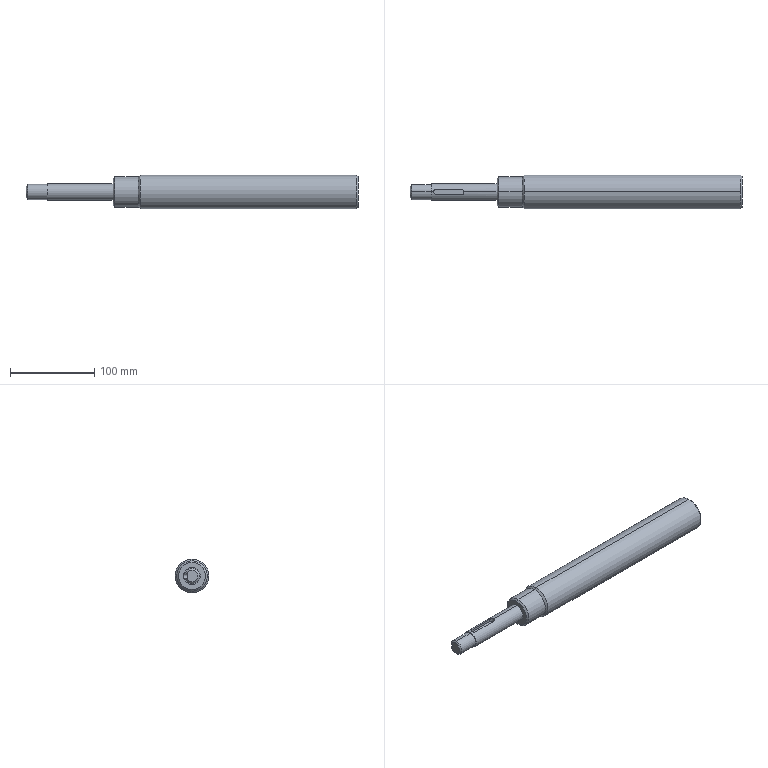Part | SolidWorks | features ICE 2, Chamfer 1, Revolution 1 | 1 solid | 32 faces | box 393 x 40 x 40 mm | volume 386098 mm3 | cylinder 13 | plane 10 | cone 9 | commonest cylinder face diameters 6 x3 18 x3 20 x2 36 x2 40 x2 5 x1
STEP:
#1=CARTESIAN_POINT('',(28.,0.,10.));
#2=VERTEX_POINT('',#1);
#3=CARTESIAN_POINT('',(31.,3.,9.539));
#4=VERTEX_POINT('',#3);
#5=CARTESIAN_POINT('',(28.,0.,10.));
#6=CARTESIAN_POINT('',(28.,0.1968,10.));
#7=CARTESIAN_POINT('',(28.02,0.3967,9.994));
#8=CARTESIAN_POINT('',(28.097,0.7821,9.971));
#9=CARTESIAN_POINT('',(28.154,0.9695,9.955));
#10=CARTESIAN_POINT('',(28.306,1.334,9.912));
#11=CARTESIAN_POINT('',(28.399,1.507,9.887));
#12=CARTESIAN_POINT('',(28.616,1.831,9.832));
#13=CARTESIAN_POINT('',(28.741,1.983,9.802));
#14=CARTESIAN_POINT('',(29.017,2.26,9.742));
#15=CARTESIAN_POINT('',(29.167,2.383,9.713));
#16=CARTESIAN_POINT('',(29.491,2.6,9.657));
#17=CARTESIAN_POINT('',(29.667,2.694,9.63));
#18=CARTESIAN_POINT('',(30.028,2.845,9.587));
#19=CARTESIAN_POINT('',(30.215,2.902,9.57));
#20=CARTESIAN_POINT('',(30.601,2.98,9.546));
#21=CARTESIAN_POINT('',(30.801,3.,9.539));
#22=CARTESIAN_POINT('',(31.,3.,9.539));
#23=B_SPLINE_CURVE_WITH_KNOTS('',3,(#5,#6,#7,#8,#9,#10,#11,#12,#13,#14,#15,#16,#17,#18,#19,#20,#21,#22),.UNSPECIFIED.,.F.,.F.,(4,2,2,2,2,2,2,2,4),(0.004718,0.005307,0.005896,0.006485,0.007074,0.007663,0.008252,0.008842,0.009431),.UNSPECIFIED.);
#24=EDGE_CURVE('',#2,#4,#23,.T.);
#25=ORIENTED_EDGE('',*,*,#24,.F.);
#26=CARTESIAN_POINT('',(28.,0.,6.5));
#27=VERTEX_POINT('',#26);
#28=CARTESIAN_POINT('',(28.,0.,20.001));
#29=DIRECTION('',(0.,0.,-1.));
#30=VECTOR('',#29,1000.);
#31=LINE('',#28,#30);
#32=EDGE_CURVE('',#2,#27,#31,.T.);
#33=ORIENTED_EDGE('',*,*,#32,.T.);
#34=CARTESIAN_POINT('',(31.,3.,6.5));
#35=VERTEX_POINT('',#34);
#36=CARTESIAN_POINT('',(31.,0.,6.5));
#37=DIRECTION('',(0.,0.,1.));
#38=DIRECTION('',(1.,0.,0.));
#39=AXIS2_PLACEMENT_3D('',#36,#37,#38);
#40=CIRCLE('',#39,3.);
#41=EDGE_CURVE('',#35,#27,#40,.T.);
#42=ORIENTED_EDGE('',*,*,#41,.F.);
#43=CARTESIAN_POINT('',(31.,3.,20.001));
#44=DIRECTION('',(0.,0.,-1.));
#45=VECTOR('',#44,1000.);
#46=LINE('',#43,#45);
#47=EDGE_CURVE('',#4,#35,#46,.T.);
#48=ORIENTED_EDGE('',*,*,#47,.F.);
#49=EDGE_LOOP('',(#25,#33,#42,#48));
#50=FACE_OUTER_BOUND('',#49,.T.);
#51=CARTESIAN_POINT('',(31.,0.,20.001));
#52=DIRECTION('',(0.,0.,-1.));
#53=DIRECTION('',(-1.,0.,0.));
#54=AXIS2_PLACEMENT_3D('',#51,#52,#53);
#55=CYLINDRICAL_SURFACE('',#54,3.);
#56=ADVANCED_FACE('',(#50),#55,.F.);
#57=CARTESIAN_POINT('',(133.,0.,18.));
#58=VERTEX_POINT('',#57);
#59=CARTESIAN_POINT('',(133.,0.,-18.));
#60=VERTEX_POINT('',#59);
#61=CARTESIAN_POINT('',(133.,0.,0.));
#62=DIRECTION('',(-1.,0.,0.));
#63=DIRECTION('',(0.,0.,1.));
#64=AXIS2_PLACEMENT_3D('',#61,#62,#63);
#65=CIRCLE('',#64,18.);
#66=EDGE_CURVE('',#58,#60,#65,.T.);
#67=ORIENTED_EDGE('',*,*,#66,.F.);
#68=CARTESIAN_POINT('',(135.,0.,20.));
#69=VERTEX_POINT('',#68);
#70=CARTESIAN_POINT('',(133.,0.,18.));
#71=DIRECTION('',(0.7071,0.,0.7071));
#72=VECTOR('',#71,1000.);
#73=LINE('',#70,#72);
#74=EDGE_CURVE('',#58,#69,#73,.T.);
#75=ORIENTED_EDGE('',*,*,#74,.T.);
#76=CARTESIAN_POINT('',(135.,0.,-20.));
#77=VERTEX_POINT('',#76);
#78=CARTESIAN_POINT('',(135.,0.,0.));
#79=DIRECTION('',(1.,0.,0.));
#80=DIRECTION('',(0.,0.,-1.));
#81=AXIS2_PLACEMENT_3D('',#78,#79,#80);
#82=CIRCLE('',#81,20.);
#83=EDGE_CURVE('',#77,#69,#82,.T.);
#84=ORIENTED_EDGE('',*,*,#83,.F.);
#85=CARTESIAN_POINT('',(133.,0.,-18.));
#86=DIRECTION('',(0.7071,0.,-0.7071));
#87=VECTOR('',#86,1000.);
#88=LINE('',#85,#87);
#89=EDGE_CURVE('',#60,#77,#88,.T.);
#90=ORIENTED_EDGE('',*,*,#89,.F.);
#91=EDGE_LOOP('',(#67,#75,#84,#90));
#92=FACE_OUTER_BOUND('',#91,.T.);
#93=CARTESIAN_POINT('',(133.,0.,0.));
#94=DIRECTION('',(1.,0.,0.));
#95=DIRECTION('',(0.,0.,-1.));
#96=AXIS2_PLACEMENT_3D('',#93,#94,#95);
#97=CONICAL_SURFACE('',#96,18.,0.7854);
#98=ADVANCED_FACE('',(#92),#97,.T.);
#99=CARTESIAN_POINT('',(103.,0.,16.));
#100=VERTEX_POINT('',#99);
#101=CARTESIAN_POINT('',(103.,0.,-16.));
#102=VERTEX_POINT('',#101);
#103=CARTESIAN_POINT('',(103.,0.,0.));
#104=DIRECTION('',(-1.,0.,0.));
#105=DIRECTION('',(0.,0.,-1.));
#106=AXIS2_PLACEMENT_3D('',#103,#104,#105);
#107=CIRCLE('',#106,16.);
#108=EDGE_CURVE('',#100,#102,#107,.T.);
#109=ORIENTED_EDGE('',*,*,#108,.F.);
#110=CARTESIAN_POINT('',(105.,0.,18.));
#111=VERTEX_POINT('',#110);
#112=CARTESIAN_POINT('',(103.,0.,16.));
#113=DIRECTION('',(0.7071,0.,0.7071));
#114=VECTOR('',#113,1000.);
#115=LINE('',#112,#114);
#116=EDGE_CURVE('',#100,#111,#115,.T.);
#117=ORIENTED_EDGE('',*,*,#116,.T.);
#118=CARTESIAN_POINT('',(105.,0.,-18.));
#119=VERTEX_POINT('',#118);
#120=CARTESIAN_POINT('',(105.,0.,0.));
#121=DIRECTION('',(1.,0.,0.));
#122=DIRECTION('',(0.,0.,-1.));
#123=AXIS2_PLACEMENT_3D('',#120,#121,#122);
#124=CIRCLE('',#123,18.);
#125=EDGE_CURVE('',#119,#111,#124,.T.);
#126=ORIENTED_EDGE('',*,*,#125,.F.);
#127=CARTESIAN_POINT('',(103.,0.,-16.));
#128=DIRECTION('',(0.7071,0.,-0.7071));
#129=VECTOR('',#128,1000.);
#130=LINE('',#127,#129);
#131=EDGE_CURVE('',#102,#119,#130,.T.);
#132=ORIENTED_EDGE('',*,*,#131,.F.);
#133=EDGE_LOOP('',(#109,#117,#126,#132));
#134=FACE_OUTER_BOUND('',#133,.T.);
#135=CARTESIAN_POINT('',(103.,0.,0.));
#136=DIRECTION('',(1.,0.,0.));
#137=DIRECTION('',(0.,0.,-1.));
#138=AXIS2_PLACEMENT_3D('',#135,#136,#137);
#139=CONICAL_SURFACE('',#138,16.,0.7854);
#140=ADVANCED_FACE('',(#134),#139,.T.);
#141=CARTESIAN_POINT('',(393.,0.,-18.));
#142=VERTEX_POINT('',#141);
#143=CARTESIAN_POINT('',(393.,0.,18.));
#144=VERTEX_POINT('',#143);
#145=CARTESIAN_POINT('',(393.,0.,0.));
#146=DIRECTION('',(1.,0.,0.));
#147=DIRECTION('',(0.,0.,1.));
#148=AXIS2_PLACEMENT_3D('',#145,#146,#147);
#149=CIRCLE('',#148,18.);
#150=EDGE_CURVE('',#142,#144,#149,.T.);
#151=ORIENTED_EDGE('',*,*,#150,.F.);
#152=CARTESIAN_POINT('',(391.,0.,-20.));
#153=VERTEX_POINT('',#152);
#154=CARTESIAN_POINT('',(391.,0.,-20.));
#155=DIRECTION('',(-0.7071,0.,-0.7071));
#156=VECTOR('',#155,1000.);
#157=LINE('',#154,#156);
#158=EDGE_CURVE('',#142,#153,#157,.T.);
#159=ORIENTED_EDGE('',*,*,#158,.T.);
#160=CARTESIAN_POINT('',(391.,0.,20.));
#161=VERTEX_POINT('',#160);
#162=CARTESIAN_POINT('',(391.,0.,0.));
#163=DIRECTION('',(-1.,0.,0.));
#164=DIRECTION('',(0.,0.,1.));
#165=AXIS2_PLACEMENT_3D('',#162,#163,#164);
#166=CIRCLE('',#165,20.);
#167=EDGE_CURVE('',#161,#153,#166,.T.);
#168=ORIENTED_EDGE('',*,*,#167,.F.);
#169=CARTESIAN_POINT('',(391.,0.,20.));
#170=DIRECTION('',(-0.7071,0.,0.7071));
#171=VECTOR('',#170,1000.);
#172=LINE('',#169,#171);
#173=EDGE_CURVE('',#144,#161,#172,.T.);
#174=ORIENTED_EDGE('',*,*,#173,.F.);
#175=EDGE_LOOP('',(#151,#159,#168,#174));
#176=FACE_OUTER_BOUND('',#175,.T.);
#177=CARTESIAN_POINT('',(391.,0.,0.));
#178=DIRECTION('',(-1.,0.,0.));
#179=DIRECTION('',(0.,0.,1.));
#180=AXIS2_PLACEMENT_3D('',#177,#178,#179);
#181=CONICAL_SURFACE('',#180,20.,0.7854);
#182=ADVANCED_FACE('',(#176),#181,.T.);
#183=ORIENTED_EDGE('',*,*,#167,.T.);
#184=CARTESIAN_POINT('',(0.,0.,-20.));
#185=DIRECTION('',(-1.,0.,0.));
#186=VECTOR('',#185,1000.);
#187=LINE('',#184,#186);
#188=EDGE_CURVE('',#153,#77,#187,.T.);
#189=ORIENTED_EDGE('',*,*,#188,.T.);
#190=ORIENTED_EDGE('',*,*,#83,.T.);
#191=CARTESIAN_POINT('',(0.,0.,20.));
#192=DIRECTION('',(-1.,0.,0.));
#193=VECTOR('',#192,1000.);
#194=LINE('',#191,#193);
#195=EDGE_CURVE('',#161,#69,#194,.T.);
#196=ORIENTED_EDGE('',*,*,#195,.F.);
#197=EDGE_LOOP('',(#183,#189,#190,#196));
#198=FACE_OUTER_BOUND('',#197,.T.);
#199=CARTESIAN_POINT('',(0.,0.,0.));
#200=DIRECTION('',(-1.,0.,0.));
#201=DIRECTION('',(0.,0.,1.));
#202=AXIS2_PLACEMENT_3D('',#199,#200,#201);
#203=CYLINDRICAL_SURFACE('',#202,20.);
#204=ADVANCED_FACE('',(#198),#203,.T.);
#205=ORIENTED_EDGE('',*,*,#66,.T.);
#206=CARTESIAN_POINT('',(0.,0.,-18.));
#207=DIRECTION('',(-1.,0.,0.));
#208=VECTOR('',#207,1000.);
#209=LINE('',#206,#208);
#210=EDGE_CURVE('',#60,#119,#209,.T.);
#211=ORIENTED_EDGE('',*,*,#210,.T.);
#212=ORIENTED_EDGE('',*,*,#125,.T.);
#213=CARTESIAN_POINT('',(0.,0.,18.));
#214=DIRECTION('',(-1.,0.,0.));
#215=VECTOR('',#214,1000.);
#216=LINE('',#213,#215);
#217=EDGE_CURVE('',#58,#111,#216,.T.);
#218=ORIENTED_EDGE('',*,*,#217,.F.);
#219=EDGE_LOOP('',(#205,#211,#212,#218));
#220=FACE_OUTER_BOUND('',#219,.T.);
#221=CARTESIAN_POINT('',(0.,0.,0.));
#222=DIRECTION('',(-1.,0.,0.));
#223=DIRECTION('',(0.,0.,1.));
#224=AXIS2_PLACEMENT_3D('',#221,#222,#223);
#225=CYLINDRICAL_SURFACE('',#224,18.);
#226=ADVANCED_FACE('',(#220),#225,.T.);
#227=CARTESIAN_POINT('',(0.,0.,7.));
#228=VERTEX_POINT('',#227);
#229=CARTESIAN_POINT('',(0.,6.538,2.5));
#230=VERTEX_POINT('',#229);
#231=CARTESIAN_POINT('',(0.,0.,0.));
#232=DIRECTION('',(-1.,0.,0.));
#233=DIRECTION('',(0.,0.,-1.));
#234=AXIS2_PLACEMENT_3D('',#231,#232,#233);
#235=CIRCLE('',#234,7.);
#236=EDGE_CURVE('',#228,#230,#235,.T.);
#237=ORIENTED_EDGE('',*,*,#236,.F.);
#238=CARTESIAN_POINT('',(2.,0.,9.));
#239=VERTEX_POINT('',#238);
#240=CARTESIAN_POINT('',(0.,0.,7.));
#241=DIRECTION('',(0.7071,0.,0.7071));
#242=VECTOR('',#241,1000.);
#243=LINE('',#240,#242);
#244=EDGE_CURVE('',#228,#239,#243,.T.);
#245=ORIENTED_EDGE('',*,*,#244,.T.);
#246=CARTESIAN_POINT('',(2.,8.646,2.5));
#247=VERTEX_POINT('',#246);
#248=CARTESIAN_POINT('',(2.,0.,0.));
#249=DIRECTION('',(1.,0.,0.));
#250=DIRECTION('',(0.,0.,-1.));
#251=AXIS2_PLACEMENT_3D('',#248,#249,#250);
#252=CIRCLE('',#251,9.);
#253=EDGE_CURVE('',#247,#239,#252,.T.);
#254=ORIENTED_EDGE('',*,*,#253,.F.);
#255=CARTESIAN_POINT('',(0.,6.538,2.5));
#256=CARTESIAN_POINT('',(0.6611,7.246,2.5));
#257=CARTESIAN_POINT('',(1.329,7.947,2.5));
#258=CARTESIAN_POINT('',(2.,8.646,2.5));
#259=B_SPLINE_CURVE_WITH_KNOTS('',3,(#255,#256,#257,#258),.UNSPECIFIED.,.F.,.F.,(4,4),(0.002866,0.005772),.UNSPECIFIED.);
#260=EDGE_CURVE('',#230,#247,#259,.T.);
#261=ORIENTED_EDGE('',*,*,#260,.F.);
#262=EDGE_LOOP('',(#237,#245,#254,#261));
#263=FACE_OUTER_BOUND('',#262,.T.);
#264=CARTESIAN_POINT('',(0.,0.,0.));
#265=DIRECTION('',(1.,0.,0.));
#266=DIRECTION('',(0.,0.,-1.));
#267=AXIS2_PLACEMENT_3D('',#264,#265,#266);
#268=CONICAL_SURFACE('',#267,7.,0.7854);
#269=ADVANCED_FACE('',(#263),#268,.T.);
#270=ORIENTED_EDGE('',*,*,#244,.F.);
#271=CARTESIAN_POINT('',(0.,0.,-7.));
#272=VERTEX_POINT('',#271);
#273=CARTESIAN_POINT('',(0.,0.,0.));
#274=DIRECTION('',(-1.,0.,0.));
#275=DIRECTION('',(0.,0.,-1.));
#276=AXIS2_PLACEMENT_3D('',#273,#274,#275);
#277=CIRCLE('',#276,7.);
#278=EDGE_CURVE('',#272,#228,#277,.T.);
#279=ORIENTED_EDGE('',*,*,#278,.F.);
#280=CARTESIAN_POINT('',(2.,0.,-9.));
#281=VERTEX_POINT('',#280);
#282=CARTESIAN_POINT('',(0.,0.,-7.));
#283=DIRECTION('',(0.7071,0.,-0.7071));
#284=VECTOR('',#283,1000.);
#285=LINE('',#282,#284);
#286=EDGE_CURVE('',#272,#281,#285,.T.);
#287=ORIENTED_EDGE('',*,*,#286,.T.);
#288=CARTESIAN_POINT('',(2.,0.,0.));
#289=DIRECTION('',(1.,0.,0.));
#290=DIRECTION('',(0.,0.,-1.));
#291=AXIS2_PLACEMENT_3D('',#288,#289,#290);
#292=CIRCLE('',#291,9.);
#293=EDGE_CURVE('',#239,#281,#292,.T.);
#294=ORIENTED_EDGE('',*,*,#293,.F.);
#295=EDGE_LOOP('',(#270,#279,#287,#294));
#296=FACE_OUTER_BOUND('',#295,.T.);
#297=CARTESIAN_POINT('',(0.,0.,0.));
#298=DIRECTION('',(1.,0.,0.));
#299=DIRECTION('',(0.,0.,-1.));
#300=AXIS2_PLACEMENT_3D('',#297,#298,#299);
#301=CONICAL_SURFACE('',#300,7.,0.7854);
#302=ADVANCED_FACE('',(#296),#301,.T.);
#303=CARTESIAN_POINT('',(25.,8.646,-2.5));
#304=VERTEX_POINT('',#303);
#305=CARTESIAN_POINT('',(25.,0.,-9.));
#306=VERTEX_POINT('',#305);
#307=CARTESIAN_POINT('',(25.,0.,0.));
#308=DIRECTION('',(-1.,0.,0.));
#309=DIRECTION('',(0.,0.,1.));
#310=AXIS2_PLACEMENT_3D('',#307,#308,#309);
#311=CIRCLE('',#310,9.);
#312=EDGE_CURVE('',#304,#306,#311,.T.);
#313=ORIENTED_EDGE('',*,*,#312,.T.);
#314=CARTESIAN_POINT('',(0.,0.,-9.));
#315=DIRECTION('',(-1.,0.,0.));
#316=VECTOR('',#315,1000.);
#317=LINE('',#314,#316);
#318=EDGE_CURVE('',#306,#281,#317,.T.);
#319=ORIENTED_EDGE('',*,*,#318,.T.);
#320=CARTESIAN_POINT('',(2.,8.646,-2.5));
#321=VERTEX_POINT('',#320);
#322=CARTESIAN_POINT('',(2.,0.,0.));
#323=DIRECTION('',(1.,0.,0.));
#324=DIRECTION('',(0.,0.,-1.));
#325=AXIS2_PLACEMENT_3D('',#322,#323,#324);
#326=CIRCLE('',#325,9.);
#327=EDGE_CURVE('',#281,#321,#326,.T.);
#328=ORIENTED_EDGE('',*,*,#327,.T.);
#329=CARTESIAN_POINT('',(0.,8.646,-2.5));
#330=DIRECTION('',(1.,0.,0.));
#331=VECTOR('',#330,1000.);
#332=LINE('',#329,#331);
#333=EDGE_CURVE('',#321,#304,#332,.T.);
#334=ORIENTED_EDGE('',*,*,#333,.T.);
#335=EDGE_LOOP('',(#313,#319,#328,#334));
#336=FACE_OUTER_BOUND('',#335,.T.);
#337=CARTESIAN_POINT('',(0.,0.,0.));
#338=DIRECTION('',(-1.,0.,0.));
#339=DIRECTION('',(0.,0.,1.));
#340=AXIS2_PLACEMENT_3D('',#337,#338,#339);
#341=CYLINDRICAL_SURFACE('',#340,9.);
#342=ADVANCED_FACE('',(#336),#341,.T.);
#343=ORIENTED_EDGE('',*,*,#318,.F.);
#344=CARTESIAN_POINT('',(25.,0.,9.));
#345=VERTEX_POINT('',#344);
#346=CARTESIAN_POINT('',(25.,0.,0.));
#347=DIRECTION('',(-1.,0.,0.));
#348=DIRECTION('',(0.,0.,1.));
#349=AXIS2_PLACEMENT_3D('',#346,#347,#348);
#350=CIRCLE('',#349,9.);
#351=EDGE_CURVE('',#306,#345,#350,.T.);
#352=ORIENTED_EDGE('',*,*,#351,.T.);
#353=CARTESIAN_POINT('',(0.,0.,9.));
#354=DIRECTION('',(-1.,0.,0.));
#355=VECTOR('',#354,1000.);
#356=LINE('',#353,#355);
#357=EDGE_CURVE('',#345,#239,#356,.T.);
#358=ORIENTED_EDGE('',*,*,#357,.T.);
#359=ORIENTED_EDGE('',*,*,#293,.T.);
#360=EDGE_LOOP('',(#343,#352,#358,#359));
#361=FACE_OUTER_BOUND('',#360,.T.);
#362=CARTESIAN_POINT('',(0.,0.,0.));
#363=DIRECTION('',(-1.,0.,0.));
#364=DIRECTION('',(0.,0.,1.));
#365=AXIS2_PLACEMENT_3D('',#362,#363,#364);
#366=CYLINDRICAL_SURFACE('',#365,9.);
#367=ADVANCED_FACE('',(#361),#366,.T.);
#368=CARTESIAN_POINT('',(103.,0.,10.));
#369=VERTEX_POINT('',#368);
#370=CARTESIAN_POINT('',(103.,0.,-10.));
#371=VERTEX_POINT('',#370);
#372=CARTESIAN_POINT('',(103.,0.,0.));
#373=DIRECTION('',(-1.,0.,0.));
#374=DIRECTION('',(0.,0.,1.));
#375=AXIS2_PLACEMENT_3D('',#372,#373,#374);
#376=CIRCLE('',#375,10.);
#377=EDGE_CURVE('',#369,#371,#376,.T.);
#378=ORIENTED_EDGE('',*,*,#377,.T.);
#379=CARTESIAN_POINT('',(25.,0.,-10.));
#380=VERTEX_POINT('',#379);
#381=CARTESIAN_POINT('',(0.,0.,-10.));
#382=DIRECTION('',(-1.,0.,0.));
#383=VECTOR('',#382,1000.);
#384=LINE('',#381,#383);
#385=EDGE_CURVE('',#371,#380,#384,.T.);
#386=ORIENTED_EDGE('',*,*,#385,.T.);
#387=CARTESIAN_POINT('',(25.,9.682,-2.5));
#388=VERTEX_POINT('',#387);
#389=CARTESIAN_POINT('',(25.,0.,0.));
#390=DIRECTION('',(-1.,0.,0.));
#391=DIRECTION('',(0.,0.,1.));
#392=AXIS2_PLACEMENT_3D('',#389,#390,#391);
#393=CIRCLE('',#392,10.);
#394=EDGE_CURVE('',#388,#380,#393,.T.);
#395=ORIENTED_EDGE('',*,*,#394,.F.);
#396=CARTESIAN_POINT('',(25.,9.682,2.5));
#397=VERTEX_POINT('',#396);
#398=CARTESIAN_POINT('',(25.,9.682,-2.5));
#399=CARTESIAN_POINT('',(25.166,9.682,-2.5));
#400=CARTESIAN_POINT('',(25.329,9.687,-2.484));
#401=CARTESIAN_POINT('',(25.649,9.703,-2.42));
#402=CARTESIAN_POINT('',(25.808,9.715,-2.371));
#403=CARTESIAN_POINT('',(26.111,9.745,-2.246));
#404=CARTESIAN_POINT('',(26.254,9.762,-2.169));
#405=CARTESIAN_POINT('',(26.525,9.801,-1.988));
#406=CARTESIAN_POINT('',(26.653,9.822,-1.883));
#407=CARTESIAN_POINT('',(26.997,9.884,-1.538));
#408=CARTESIAN_POINT('',(27.183,9.925,-1.26));
#409=CARTESIAN_POINT('',(27.371,9.968,-0.8098));
#410=CARTESIAN_POINT('',(27.419,9.98,-0.6515));
#411=CARTESIAN_POINT('',(27.484,9.996,-0.3286));
#412=CARTESIAN_POINT('',(27.5,10.,-0.166));
#413=CARTESIAN_POINT('',(27.5,10.,0.1615));
#414=CARTESIAN_POINT('',(27.484,9.996,0.3279));
#415=CARTESIAN_POINT('',(27.42,9.98,0.649));
#416=CARTESIAN_POINT('',(27.372,9.969,0.8052));
#417=CARTESIAN_POINT('',(27.184,9.925,1.26));
#418=CARTESIAN_POINT('',(27.,9.884,1.535));
#419=CARTESIAN_POINT('',(26.653,9.822,1.883));
#420=CARTESIAN_POINT('',(26.527,9.801,1.986));
#421=CARTESIAN_POINT('',(26.257,9.763,2.167));
#422=CARTESIAN_POINT('',(26.111,9.745,2.246));
#423=CARTESIAN_POINT('',(25.809,9.715,2.371));
#424=CARTESIAN_POINT('',(25.654,9.703,2.419));
#425=CARTESIAN_POINT('',(25.332,9.687,2.483));
#426=CARTESIAN_POINT('',(25.166,9.682,2.5));
#427=CARTESIAN_POINT('',(25.,9.682,2.5));
#428=B_SPLINE_CURVE_WITH_KNOTS('',3,(#398,#399,#400,#401,#402,#403,#404,#405,#406,#407,#408,#409,#410,#411,#412,#413,#414,#415,#416,#417,#418,#419,#420,#421,#422,#423,#424,#425,#426,#427),.UNSPECIFIED.,.F.,.F.,(4,2,2,2,2,2,2,2,2,2,2,2,2,2,4),(0.,0.0004903,0.0009806,0.001471,0.001961,0.002942,0.003432,0.003922,0.004413,0.004903,0.005884,0.006374,0.006864,0.007355,0.007845),.UNSPECIFIED.);
#429=EDGE_CURVE('',#388,#397,#428,.T.);
#430=ORIENTED_EDGE('',*,*,#429,.T.);
#431=CARTESIAN_POINT('',(25.,0.,10.));
#432=VERTEX_POINT('',#431);
#433=CARTESIAN_POINT('',(25.,0.,0.));
#434=DIRECTION('',(-1.,0.,0.));
#435=DIRECTION('',(0.,0.,1.));
#436=AXIS2_PLACEMENT_3D('',#433,#434,#435);
#437=CIRCLE('',#436,10.);
#438=EDGE_CURVE('',#432,#397,#437,.T.);
#439=ORIENTED_EDGE('',*,*,#438,.F.);
#440=CARTESIAN_POINT('',(0.,0.,10.));
#441=DIRECTION('',(-1.,0.,0.));
#442=VECTOR('',#441,1000.);
#443=LINE('',#440,#442);
#444=EDGE_CURVE('',#2,#432,#443,.T.);
#445=ORIENTED_EDGE('',*,*,#444,.F.);
#446=ORIENTED_EDGE('',*,*,#24,.T.);
#447=CARTESIAN_POINT('',(61.,3.,9.539));
#448=VERTEX_POINT('',#447);
#449=CARTESIAN_POINT('',(0.,3.,9.539));
#450=DIRECTION('',(1.,0.,0.));
#451=VECTOR('',#450,1000.);
#452=LINE('',#449,#451);
#453=EDGE_CURVE('',#4,#448,#452,.T.);
#454=ORIENTED_EDGE('',*,*,#453,.T.);
#455=CARTESIAN_POINT('',(64.,0.,10.));
#456=VERTEX_POINT('',#455);
#457=CARTESIAN_POINT('',(61.,3.,9.539));
#458=CARTESIAN_POINT('',(61.2,3.,9.539));
#459=CARTESIAN_POINT('',(61.395,2.98,9.546));
#460=CARTESIAN_POINT('',(61.781,2.903,9.569));
#461=CARTESIAN_POINT('',(61.972,2.845,9.587));
#462=CARTESIAN_POINT('',(62.335,2.694,9.631));
#463=CARTESIAN_POINT('',(62.506,2.602,9.656));
#464=CARTESIAN_POINT('',(62.832,2.384,9.712));
#465=CARTESIAN_POINT('',(62.985,2.258,9.743));
#466=CARTESIAN_POINT('',(63.397,1.845,9.832));
#467=CARTESIAN_POINT('',(63.62,1.512,9.892));
#468=CARTESIAN_POINT('',(63.845,0.971,9.954));
#469=CARTESIAN_POINT('',(63.903,0.7806,9.971));
#470=CARTESIAN_POINT('',(63.981,0.3926,9.994));
#471=CARTESIAN_POINT('',(64.,0.197,10.));
#472=CARTESIAN_POINT('',(64.,0.,10.));
#473=B_SPLINE_CURVE_WITH_KNOTS('',3,(#457,#458,#459,#460,#461,#462,#463,#464,#465,#466,#467,#468,#469,#470,#471,#472),.UNSPECIFIED.,.F.,.F.,(4,2,2,2,2,2,2,4),(0.,0.0005898,0.00118,0.001769,0.002359,0.003539,0.004128,0.004718),.UNSPECIFIED.);
#474=EDGE_CURVE('',#448,#456,#473,.T.);
#475=ORIENTED_EDGE('',*,*,#474,.T.);
#476=CARTESIAN_POINT('',(0.,0.,10.));
#477=DIRECTION('',(-1.,0.,0.));
#478=VECTOR('',#477,1000.);
#479=LINE('',#476,#478);
#480=EDGE_CURVE('',#369,#456,#479,.T.);
#481=ORIENTED_EDGE('',*,*,#480,.F.);
#482=EDGE_LOOP('',(#378,#386,#395,#430,#439,#445,#446,#454,#475,#481));
#483=FACE_OUTER_BOUND('',#482,.T.);
#484=CARTESIAN_POINT('',(0.,0.,0.));
#485=DIRECTION('',(-1.,0.,0.));
#486=DIRECTION('',(0.,0.,1.));
#487=AXIS2_PLACEMENT_3D('',#484,#485,#486);
#488=CYLINDRICAL_SURFACE('',#487,10.);
#489=ADVANCED_FACE('',(#483),#488,.T.);
#490=ORIENTED_EDGE('',*,*,#385,.F.);
#491=CARTESIAN_POINT('',(103.,0.,0.));
#492=DIRECTION('',(-1.,0.,0.));
#493=DIRECTION('',(0.,0.,1.));
#494=AXIS2_PLACEMENT_3D('',#491,#492,#493);
#495=CIRCLE('',#494,10.);
#496=EDGE_CURVE('',#371,#369,#495,.T.);
#497=ORIENTED_EDGE('',*,*,#496,.T.);
#498=ORIENTED_EDGE('',*,*,#480,.T.);
#499=CARTESIAN_POINT('',(61.,-3.,9.539));
#500=VERTEX_POINT('',#499);
#501=CARTESIAN_POINT('',(64.,0.,10.));
#502=CARTESIAN_POINT('',(64.,-0.1968,10.));
#503=CARTESIAN_POINT('',(63.98,-0.3967,9.994));
#504=CARTESIAN_POINT('',(63.903,-0.7821,9.971));
#505=CARTESIAN_POINT('',(63.846,-0.9695,9.955));
#506=CARTESIAN_POINT('',(63.694,-1.334,9.912));
#507=CARTESIAN_POINT('',(63.601,-1.507,9.887));
#508=CARTESIAN_POINT('',(63.384,-1.831,9.832));
#509=CARTESIAN_POINT('',(63.259,-1.983,9.802));
#510=CARTESIAN_POINT('',(62.983,-2.26,9.742));
#511=CARTESIAN_POINT('',(62.833,-2.383,9.713));
#512=CARTESIAN_POINT('',(62.509,-2.6,9.657));
#513=CARTESIAN_POINT('',(62.333,-2.694,9.63));
#514=CARTESIAN_POINT('',(61.972,-2.845,9.587));
#515=CARTESIAN_POINT('',(61.785,-2.902,9.57));
#516=CARTESIAN_POINT('',(61.399,-2.98,9.546));
#517=CARTESIAN_POINT('',(61.199,-3.,9.539));
#518=CARTESIAN_POINT('',(61.,-3.,9.539));
#519=B_SPLINE_CURVE_WITH_KNOTS('',3,(#501,#502,#503,#504,#505,#506,#507,#508,#509,#510,#511,#512,#513,#514,#515,#516,#517,#518),.UNSPECIFIED.,.F.,.F.,(4,2,2,2,2,2,2,2,4),(0.004718,0.005307,0.005896,0.006485,0.007074,0.007663,0.008252,0.008842,0.009431),.UNSPECIFIED.);
#520=EDGE_CURVE('',#456,#500,#519,.T.);
#521=ORIENTED_EDGE('',*,*,#520,.T.);
#522=CARTESIAN_POINT('',(31.,-3.,9.539));
#523=VERTEX_POINT('',#522);
#524=CARTESIAN_POINT('',(0.,-3.,9.539));
#525=DIRECTION('',(-1.,0.,0.));
#526=VECTOR('',#525,1000.);
#527=LINE('',#524,#526);
#528=EDGE_CURVE('',#500,#523,#527,.T.);
#529=ORIENTED_EDGE('',*,*,#528,.T.);
#530=CARTESIAN_POINT('',(31.,-3.,9.539));
#531=CARTESIAN_POINT('',(30.8,-3.,9.539));
#532=CARTESIAN_POINT('',(30.605,-2.98,9.546));
#533=CARTESIAN_POINT('',(30.219,-2.903,9.569));
#534=CARTESIAN_POINT('',(30.028,-2.845,9.587));
#535=CARTESIAN_POINT('',(29.665,-2.694,9.631));
#536=CARTESIAN_POINT('',(29.494,-2.602,9.656));
#537=CARTESIAN_POINT('',(29.168,-2.384,9.712));
#538=CARTESIAN_POINT('',(29.015,-2.258,9.743));
#539=CARTESIAN_POINT('',(28.603,-1.845,9.832));
#540=CARTESIAN_POINT('',(28.38,-1.512,9.892));
#541=CARTESIAN_POINT('',(28.155,-0.971,9.954));
#542=CARTESIAN_POINT('',(28.097,-0.7806,9.971));
#543=CARTESIAN_POINT('',(28.019,-0.3926,9.994));
#544=CARTESIAN_POINT('',(28.,-0.197,10.));
#545=CARTESIAN_POINT('',(28.,0.,10.));
#546=B_SPLINE_CURVE_WITH_KNOTS('',3,(#530,#531,#532,#533,#534,#535,#536,#537,#538,#539,#540,#541,#542,#543,#544,#545),.UNSPECIFIED.,.F.,.F.,(4,2,2,2,2,2,2,4),(0.,0.0005898,0.00118,0.001769,0.002359,0.003539,0.004128,0.004718),.UNSPECIFIED.);
#547=EDGE_CURVE('',#523,#2,#546,.T.);
#548=ORIENTED_EDGE('',*,*,#547,.T.);
#549=ORIENTED_EDGE('',*,*,#444,.T.);
#550=CARTESIAN_POINT('',(25.,0.,0.));
#551=DIRECTION('',(-1.,0.,0.));
#552=DIRECTION('',(0.,0.,1.));
#553=AXIS2_PLACEMENT_3D('',#550,#551,#552);
#554=CIRCLE('',#553,10.);
#555=EDGE_CURVE('',#380,#432,#554,.T.);
#556=ORIENTED_EDGE('',*,*,#555,.F.);
#557=EDGE_LOOP('',(#490,#497,#498,#521,#529,#548,#549,#556));
#558=FACE_OUTER_BOUND('',#557,.T.);
#559=CARTESIAN_POINT('',(0.,0.,0.));
#560=DIRECTION('',(-1.,0.,0.));
#561=DIRECTION('',(0.,0.,1.));
#562=AXIS2_PLACEMENT_3D('',#559,#560,#561);
#563=CYLINDRICAL_SURFACE('',#562,10.);
#564=ADVANCED_FACE('',(#558),#563,.T.);
#565=CARTESIAN_POINT('',(0.,5.,2.5));
#566=VERTEX_POINT('',#565);
#567=CARTESIAN_POINT('',(0.,20.001,2.5));
#568=DIRECTION('',(0.,-1.,0.));
#569=VECTOR('',#568,1000.);
#570=LINE('',#567,#569);
#571=EDGE_CURVE('',#230,#566,#570,.T.);
#572=ORIENTED_EDGE('',*,*,#571,.T.);
#573=CARTESIAN_POINT('',(0.,5.,-2.5));
#574=VERTEX_POINT('',#573);
#575=CARTESIAN_POINT('',(0.,5.,0.));
#576=DIRECTION('',(0.,0.,-1.));
#577=VECTOR('',#576,1000.);
#578=LINE('',#575,#577);
#579=EDGE_CURVE('',#566,#574,#578,.T.);
#580=ORIENTED_EDGE('',*,*,#579,.T.);
#581=CARTESIAN_POINT('',(0.,6.538,-2.5));
#582=VERTEX_POINT('',#581);
#583=CARTESIAN_POINT('',(0.,20.001,-2.5));
#584=DIRECTION('',(0.,1.,0.));
#585=VECTOR('',#584,1000.);
#586=LINE('',#583,#585);
#587=EDGE_CURVE('',#574,#582,#586,.T.);
#588=ORIENTED_EDGE('',*,*,#587,.T.);
#589=CARTESIAN_POINT('',(0.,0.,0.));
#590=DIRECTION('',(-1.,0.,0.));
#591=DIRECTION('',(0.,0.,-1.));
#592=AXIS2_PLACEMENT_3D('',#589,#590,#591);
#593=CIRCLE('',#592,7.);
#594=EDGE_CURVE('',#582,#272,#593,.T.);
#595=ORIENTED_EDGE('',*,*,#594,.T.);
#596=ORIENTED_EDGE('',*,*,#278,.T.);
#597=ORIENTED_EDGE('',*,*,#236,.T.);
#598=EDGE_LOOP('',(#572,#580,#588,#595,#596,#597));
#599=FACE_OUTER_BOUND('',#598,.T.);
#600=CARTESIAN_POINT('',(0.,0.,0.));
#601=DIRECTION('',(1.,0.,0.));
#602=DIRECTION('',(0.,0.,-1.));
#603=AXIS2_PLACEMENT_3D('',#600,#601,#602);
#604=PLANE('',#603);
#605=ADVANCED_FACE('',(#599),#604,.F.);
#606=ORIENTED_EDGE('',*,*,#357,.F.);
#607=CARTESIAN_POINT('',(25.,8.646,2.5));
#608=VERTEX_POINT('',#607);
#609=CARTESIAN_POINT('',(25.,0.,0.));
#610=DIRECTION('',(-1.,0.,0.));
#611=DIRECTION('',(0.,0.,1.));
#612=AXIS2_PLACEMENT_3D('',#609,#610,#611);
#613=CIRCLE('',#612,9.);
#614=EDGE_CURVE('',#345,#608,#613,.T.);
#615=ORIENTED_EDGE('',*,*,#614,.T.);
#616=CARTESIAN_POINT('',(0.,8.646,2.5));
#617=DIRECTION('',(-1.,0.,0.));
#618=VECTOR('',#617,1000.);
#619=LINE('',#616,#618);
#620=EDGE_CURVE('',#608,#247,#619,.T.);
#621=ORIENTED_EDGE('',*,*,#620,.T.);
#622=ORIENTED_EDGE('',*,*,#253,.T.);
#623=EDGE_LOOP('',(#606,#615,#621,#622));
#624=FACE_OUTER_BOUND('',#623,.T.);
#625=CARTESIAN_POINT('',(0.,0.,0.));
#626=DIRECTION('',(-1.,0.,0.));
#627=DIRECTION('',(0.,0.,1.));
#628=AXIS2_PLACEMENT_3D('',#625,#626,#627);
#629=CYLINDRICAL_SURFACE('',#628,9.);
#630=ADVANCED_FACE('',(#624),#629,.T.);
#631=CARTESIAN_POINT('',(25.,20.001,2.5));
#632=DIRECTION('',(0.,-1.,0.));
#633=VECTOR('',#632,1000.);
#634=LINE('',#631,#633);
#635=EDGE_CURVE('',#397,#608,#634,.T.);
#636=ORIENTED_EDGE('',*,*,#635,.T.);
#637=ORIENTED_EDGE('',*,*,#614,.F.);
#638=ORIENTED_EDGE('',*,*,#351,.F.);
#639=ORIENTED_EDGE('',*,*,#312,.F.);
#640=CARTESIAN_POINT('',(25.,20.001,-2.5));
#641=DIRECTION('',(0.,-1.,0.));
#642=VECTOR('',#641,1000.);
#643=LINE('',#640,#642);
#644=EDGE_CURVE('',#388,#304,#643,.T.);
#645=ORIENTED_EDGE('',*,*,#644,.F.);
#646=ORIENTED_EDGE('',*,*,#394,.T.);
#647=ORIENTED_EDGE('',*,*,#555,.T.);
#648=ORIENTED_EDGE('',*,*,#438,.T.);
#649=EDGE_LOOP('',(#636,#637,#638,#639,#645,#646,#647,#648));
#650=FACE_OUTER_BOUND('',#649,.T.);
#651=CARTESIAN_POINT('',(25.,9.,0.));
#652=DIRECTION('',(1.,0.,0.));
#653=DIRECTION('',(0.,0.,-1.));
#654=AXIS2_PLACEMENT_3D('',#651,#652,#653);
#655=PLANE('',#654);
#656=ADVANCED_FACE('',(#650),#655,.F.);
#657=ORIENTED_EDGE('',*,*,#286,.F.);
#658=ORIENTED_EDGE('',*,*,#594,.F.);
#659=CARTESIAN_POINT('',(2.,8.646,-2.5));
#660=CARTESIAN_POINT('',(1.329,7.947,-2.5));
#661=CARTESIAN_POINT('',(0.6611,7.246,-2.5));
#662=CARTESIAN_POINT('',(0.,6.538,-2.5));
#663=B_SPLINE_CURVE_WITH_KNOTS('',3,(#659,#660,#661,#662),.UNSPECIFIED.,.F.,.F.,(4,4),(0.00629,0.009196),.UNSPECIFIED.);
#664=EDGE_CURVE('',#321,#582,#663,.T.);
#665=ORIENTED_EDGE('',*,*,#664,.F.);
#666=ORIENTED_EDGE('',*,*,#327,.F.);
#667=EDGE_LOOP('',(#657,#658,#665,#666));
#668=FACE_OUTER_BOUND('',#667,.T.);
#669=CARTESIAN_POINT('',(0.,0.,0.));
#670=DIRECTION('',(1.,0.,0.));
#671=DIRECTION('',(0.,0.,-1.));
#672=AXIS2_PLACEMENT_3D('',#669,#670,#671);
#673=CONICAL_SURFACE('',#672,7.,0.7854);
#674=ADVANCED_FACE('',(#668),#673,.T.);
#675=CARTESIAN_POINT('',(103.,0.,0.));
#676=DIRECTION('',(-1.,0.,0.));
#677=DIRECTION('',(0.,0.,-1.));
#678=AXIS2_PLACEMENT_3D('',#675,#676,#677);
#679=CIRCLE('',#678,16.);
#680=EDGE_CURVE('',#102,#100,#679,.T.);
#681=ORIENTED_EDGE('',*,*,#680,.T.);
#682=ORIENTED_EDGE('',*,*,#108,.T.);
#683=EDGE_LOOP('',(#681,#682));
#684=FACE_OUTER_BOUND('',#683,.T.);
#685=ORIENTED_EDGE('',*,*,#377,.F.);
#686=ORIENTED_EDGE('',*,*,#496,.F.);
#687=EDGE_LOOP('',(#685,#686));
#688=FACE_BOUND('',#687,.T.);
#689=CARTESIAN_POINT('',(103.,10.,0.));
#690=DIRECTION('',(1.,0.,0.));
#691=DIRECTION('',(0.,0.,-1.));
#692=AXIS2_PLACEMENT_3D('',#689,#690,#691);
#693=PLANE('',#692);
#694=ADVANCED_FACE('',(#684,#688),#693,.F.);
#695=ORIENTED_EDGE('',*,*,#210,.F.);
#696=CARTESIAN_POINT('',(133.,0.,0.));
#697=DIRECTION('',(-1.,0.,0.));
#698=DIRECTION('',(0.,0.,1.));
#699=AXIS2_PLACEMENT_3D('',#696,#697,#698);
#700=CIRCLE('',#699,18.);
#701=EDGE_CURVE('',#60,#58,#700,.T.);
#702=ORIENTED_EDGE('',*,*,#701,.T.);
#703=ORIENTED_EDGE('',*,*,#217,.T.);
#704=CARTESIAN_POINT('',(105.,0.,0.));
#705=DIRECTION('',(1.,0.,0.));
#706=DIRECTION('',(0.,0.,-1.));
#707=AXIS2_PLACEMENT_3D('',#704,#705,#706);
#708=CIRCLE('',#707,18.);
#709=EDGE_CURVE('',#111,#119,#708,.T.);
#710=ORIENTED_EDGE('',*,*,#709,.T.);
#711=EDGE_LOOP('',(#695,#702,#703,#710));
#712=FACE_OUTER_BOUND('',#711,.T.);
#713=CARTESIAN_POINT('',(0.,0.,0.));
#714=DIRECTION('',(-1.,0.,0.));
#715=DIRECTION('',(0.,0.,1.));
#716=AXIS2_PLACEMENT_3D('',#713,#714,#715);
#717=CYLINDRICAL_SURFACE('',#716,18.);
#718=ADVANCED_FACE('',(#712),#717,.T.);
#719=ORIENTED_EDGE('',*,*,#188,.F.);
#720=CARTESIAN_POINT('',(391.,0.,0.));
#721=DIRECTION('',(-1.,0.,0.));
#722=DIRECTION('',(0.,0.,1.));
#723=AXIS2_PLACEMENT_3D('',#720,#721,#722);
#724=CIRCLE('',#723,20.);
#725=EDGE_CURVE('',#153,#161,#724,.T.);
#726=ORIENTED_EDGE('',*,*,#725,.T.);
#727=ORIENTED_EDGE('',*,*,#195,.T.);
#728=CARTESIAN_POINT('',(135.,0.,0.));
#729=DIRECTION('',(1.,0.,0.));
#730=DIRECTION('',(0.,0.,-1.));
#731=AXIS2_PLACEMENT_3D('',#728,#729,#730);
#732=CIRCLE('',#731,20.);
#733=EDGE_CURVE('',#69,#77,#732,.T.);
#734=ORIENTED_EDGE('',*,*,#733,.T.);
#735=EDGE_LOOP('',(#719,#726,#727,#734));
#736=FACE_OUTER_BOUND('',#735,.T.);
#737=CARTESIAN_POINT('',(0.,0.,0.));
#738=DIRECTION('',(-1.,0.,0.));
#739=DIRECTION('',(0.,0.,1.));
#740=AXIS2_PLACEMENT_3D('',#737,#738,#739);
#741=CYLINDRICAL_SURFACE('',#740,20.);
#742=ADVANCED_FACE('',(#736),#741,.T.);
#743=CARTESIAN_POINT('',(393.,0.,0.));
#744=DIRECTION('',(1.,0.,0.));
#745=DIRECTION('',(0.,0.,1.));
#746=AXIS2_PLACEMENT_3D('',#743,#744,#745);
#747=CIRCLE('',#746,18.);
#748=EDGE_CURVE('',#144,#142,#747,.T.);
#749=ORIENTED_EDGE('',*,*,#748,.T.);
#750=ORIENTED_EDGE('',*,*,#150,.T.);
#751=EDGE_LOOP('',(#749,#750));
#752=FACE_OUTER_BOUND('',#751,.T.);
#753=CARTESIAN_POINT('',(393.,20.,0.));
#754=DIRECTION('',(-1.,0.,0.));
#755=DIRECTION('',(0.,0.,1.));
#756=AXIS2_PLACEMENT_3D('',#753,#754,#755);
#757=PLANE('',#756);
#758=ADVANCED_FACE('',(#752),#757,.F.);
#759=ORIENTED_EDGE('',*,*,#158,.F.);
#760=ORIENTED_EDGE('',*,*,#748,.F.);
#761=ORIENTED_EDGE('',*,*,#173,.T.);
#762=ORIENTED_EDGE('',*,*,#725,.F.);
#763=EDGE_LOOP('',(#759,#760,#761,#762));
#764=FACE_OUTER_BOUND('',#763,.T.);
#765=CARTESIAN_POINT('',(391.,0.,0.));
#766=DIRECTION('',(-1.,0.,0.));
#767=DIRECTION('',(0.,0.,1.));
#768=AXIS2_PLACEMENT_3D('',#765,#766,#767);
#769=CONICAL_SURFACE('',#768,20.,0.7854);
#770=ADVANCED_FACE('',(#764),#769,.T.);
#771=ORIENTED_EDGE('',*,*,#116,.F.);
#772=ORIENTED_EDGE('',*,*,#680,.F.);
#773=ORIENTED_EDGE('',*,*,#131,.T.);
#774=ORIENTED_EDGE('',*,*,#709,.F.);
#775=EDGE_LOOP('',(#771,#772,#773,#774));
#776=FACE_OUTER_BOUND('',#775,.T.);
#777=CARTESIAN_POINT('',(103.,0.,0.));
#778=DIRECTION('',(1.,0.,0.));
#779=DIRECTION('',(0.,0.,-1.));
#780=AXIS2_PLACEMENT_3D('',#777,#778,#779);
#781=CONICAL_SURFACE('',#780,16.,0.7854);
#782=ADVANCED_FACE('',(#776),#781,.T.);
#783=ORIENTED_EDGE('',*,*,#74,.F.);
#784=ORIENTED_EDGE('',*,*,#701,.F.);
#785=ORIENTED_EDGE('',*,*,#89,.T.);
#786=ORIENTED_EDGE('',*,*,#733,.F.);
#787=EDGE_LOOP('',(#783,#784,#785,#786));
#788=FACE_OUTER_BOUND('',#787,.T.);
#789=CARTESIAN_POINT('',(133.,0.,0.));
#790=DIRECTION('',(1.,0.,0.));
#791=DIRECTION('',(0.,0.,-1.));
#792=AXIS2_PLACEMENT_3D('',#789,#790,#791);
#793=CONICAL_SURFACE('',#792,18.,0.7854);
#794=ADVANCED_FACE('',(#788),#793,.T.);
#795=ORIENTED_EDGE('',*,*,#32,.F.);
#796=ORIENTED_EDGE('',*,*,#547,.F.);
#797=CARTESIAN_POINT('',(31.,-3.,6.5));
#798=VERTEX_POINT('',#797);
#799=CARTESIAN_POINT('',(31.,-3.,20.001));
#800=DIRECTION('',(0.,0.,-1.));
#801=VECTOR('',#800,1000.);
#802=LINE('',#799,#801);
#803=EDGE_CURVE('',#523,#798,#802,.T.);
#804=ORIENTED_EDGE('',*,*,#803,.T.);
#805=CARTESIAN_POINT('',(31.,0.,6.5));
#806=DIRECTION('',(0.,0.,1.));
#807=DIRECTION('',(1.,0.,0.));
#808=AXIS2_PLACEMENT_3D('',#805,#806,#807);
#809=CIRCLE('',#808,3.);
#810=EDGE_CURVE('',#27,#798,#809,.T.);
#811=ORIENTED_EDGE('',*,*,#810,.F.);
#812=EDGE_LOOP('',(#795,#796,#804,#811));
#813=FACE_OUTER_BOUND('',#812,.T.);
#814=CARTESIAN_POINT('',(31.,0.,20.001));
#815=DIRECTION('',(0.,0.,-1.));
#816=DIRECTION('',(-1.,0.,0.));
#817=AXIS2_PLACEMENT_3D('',#814,#815,#816);
#818=CYLINDRICAL_SURFACE('',#817,3.);
#819=ADVANCED_FACE('',(#813),#818,.F.);
#820=CARTESIAN_POINT('',(61.,-3.,6.5));
#821=VERTEX_POINT('',#820);
#822=CARTESIAN_POINT('',(61.,-3.,20.001));
#823=DIRECTION('',(0.,0.,-1.));
#824=VECTOR('',#823,1000.);
#825=LINE('',#822,#824);
#826=EDGE_CURVE('',#500,#821,#825,.T.);
#827=ORIENTED_EDGE('',*,*,#826,.T.);
#828=CARTESIAN_POINT('',(31.,-3.,6.5));
#829=DIRECTION('',(1.,0.,0.));
#830=VECTOR('',#829,1000.);
#831=LINE('',#828,#830);
#832=EDGE_CURVE('',#798,#821,#831,.T.);
#833=ORIENTED_EDGE('',*,*,#832,.F.);
#834=ORIENTED_EDGE('',*,*,#803,.F.);
#835=ORIENTED_EDGE('',*,*,#528,.F.);
#836=EDGE_LOOP('',(#827,#833,#834,#835));
#837=FACE_OUTER_BOUND('',#836,.T.);
#838=CARTESIAN_POINT('',(31.,-3.,20.001));
#839=DIRECTION('',(0.,1.,0.));
#840=DIRECTION('',(0.,0.,1.));
#841=AXIS2_PLACEMENT_3D('',#838,#839,#840);
#842=PLANE('',#841);
#843=ADVANCED_FACE('',(#837),#842,.T.);
#844=CARTESIAN_POINT('',(61.,3.,6.5));
#845=VERTEX_POINT('',#844);
#846=CARTESIAN_POINT('',(61.,3.,20.001));
#847=DIRECTION('',(0.,0.,-1.));
#848=VECTOR('',#847,1000.);
#849=LINE('',#846,#848);
#850=EDGE_CURVE('',#448,#845,#849,.T.);
#851=ORIENTED_EDGE('',*,*,#850,.T.);
#852=CARTESIAN_POINT('',(61.,0.,6.5));
#853=DIRECTION('',(0.,0.,1.));
#854=DIRECTION('',(1.,0.,0.));
#855=AXIS2_PLACEMENT_3D('',#852,#853,#854);
#856=CIRCLE('',#855,3.);
#857=EDGE_CURVE('',#821,#845,#856,.T.);
#858=ORIENTED_EDGE('',*,*,#857,.F.);
#859=ORIENTED_EDGE('',*,*,#826,.F.);
#860=ORIENTED_EDGE('',*,*,#520,.F.);
#861=ORIENTED_EDGE('',*,*,#474,.F.);
#862=EDGE_LOOP('',(#851,#858,#859,#860,#861));
#863=FACE_OUTER_BOUND('',#862,.T.);
#864=CARTESIAN_POINT('',(61.,0.,20.001));
#865=DIRECTION('',(0.,0.,-1.));
#866=DIRECTION('',(-1.,0.,0.));
#867=AXIS2_PLACEMENT_3D('',#864,#865,#866);
#868=CYLINDRICAL_SURFACE('',#867,3.);
#869=ADVANCED_FACE('',(#863),#868,.F.);
#870=ORIENTED_EDGE('',*,*,#47,.T.);
#871=CARTESIAN_POINT('',(31.,3.,6.5));
#872=DIRECTION('',(-1.,0.,0.));
#873=VECTOR('',#872,1000.);
#874=LINE('',#871,#873);
#875=EDGE_CURVE('',#845,#35,#874,.T.);
#876=ORIENTED_EDGE('',*,*,#875,.F.);
#877=ORIENTED_EDGE('',*,*,#850,.F.);
#878=ORIENTED_EDGE('',*,*,#453,.F.);
#879=EDGE_LOOP('',(#870,#876,#877,#878));
#880=FACE_OUTER_BOUND('',#879,.T.);
#881=CARTESIAN_POINT('',(31.,3.,20.001));
#882=DIRECTION('',(0.,-1.,0.));
#883=DIRECTION('',(0.,0.,-1.));
#884=AXIS2_PLACEMENT_3D('',#881,#882,#883);
#885=PLANE('',#884);
#886=ADVANCED_FACE('',(#880),#885,.T.);
#887=ORIENTED_EDGE('',*,*,#41,.T.);
#888=ORIENTED_EDGE('',*,*,#810,.T.);
#889=ORIENTED_EDGE('',*,*,#832,.T.);
#890=ORIENTED_EDGE('',*,*,#857,.T.);
#891=ORIENTED_EDGE('',*,*,#875,.T.);
#892=EDGE_LOOP('',(#887,#888,#889,#890,#891));
#893=FACE_OUTER_BOUND('',#892,.T.);
#894=CARTESIAN_POINT('',(31.,0.,6.5));
#895=DIRECTION('',(0.,0.,1.));
#896=DIRECTION('',(1.,0.,0.));
#897=AXIS2_PLACEMENT_3D('',#894,#895,#896);
#898=PLANE('',#897);
#899=ADVANCED_FACE('',(#893),#898,.T.);
#900=CARTESIAN_POINT('',(25.,5.,2.5));
#901=VERTEX_POINT('',#900);
#902=CARTESIAN_POINT('',(25.,20.001,2.5));
#903=DIRECTION('',(0.,-1.,0.));
#904=VECTOR('',#903,1000.);
#905=LINE('',#902,#904);
#906=EDGE_CURVE('',#608,#901,#905,.T.);
#907=ORIENTED_EDGE('',*,*,#906,.T.);
#908=CARTESIAN_POINT('',(0.,5.,2.5));
#909=DIRECTION('',(1.,0.,0.));
#910=VECTOR('',#909,1000.);
#911=LINE('',#908,#910);
#912=EDGE_CURVE('',#566,#901,#911,.T.);
#913=ORIENTED_EDGE('',*,*,#912,.F.);
#914=ORIENTED_EDGE('',*,*,#571,.F.);
#915=ORIENTED_EDGE('',*,*,#260,.T.);
#916=ORIENTED_EDGE('',*,*,#620,.F.);
#917=EDGE_LOOP('',(#907,#913,#914,#915,#916));
#918=FACE_OUTER_BOUND('',#917,.T.);
#919=CARTESIAN_POINT('',(0.,20.001,2.5));
#920=DIRECTION('',(0.,0.,-1.));
#921=DIRECTION('',(-1.,0.,0.));
#922=AXIS2_PLACEMENT_3D('',#919,#920,#921);
#923=PLANE('',#922);
#924=ADVANCED_FACE('',(#918),#923,.T.);
#925=ORIENTED_EDGE('',*,*,#644,.T.);
#926=CARTESIAN_POINT('',(25.,5.,-2.5));
#927=VERTEX_POINT('',#926);
#928=CARTESIAN_POINT('',(25.,20.001,-2.5));
#929=DIRECTION('',(0.,-1.,0.));
#930=VECTOR('',#929,1000.);
#931=LINE('',#928,#930);
#932=EDGE_CURVE('',#304,#927,#931,.T.);
#933=ORIENTED_EDGE('',*,*,#932,.T.);
#934=CARTESIAN_POINT('',(25.,5.,0.));
#935=DIRECTION('',(0.,1.,0.));
#936=DIRECTION('',(0.,0.,1.));
#937=AXIS2_PLACEMENT_3D('',#934,#935,#936);
#938=CIRCLE('',#937,2.5);
#939=EDGE_CURVE('',#901,#927,#938,.T.);
#940=ORIENTED_EDGE('',*,*,#939,.F.);
#941=ORIENTED_EDGE('',*,*,#906,.F.);
#942=ORIENTED_EDGE('',*,*,#635,.F.);
#943=ORIENTED_EDGE('',*,*,#429,.F.);
#944=EDGE_LOOP('',(#925,#933,#940,#941,#942,#943));
#945=FACE_OUTER_BOUND('',#944,.T.);
#946=CARTESIAN_POINT('',(25.,20.001,0.));
#947=DIRECTION('',(0.,-1.,0.));
#948=DIRECTION('',(0.,0.,-1.));
#949=AXIS2_PLACEMENT_3D('',#946,#947,#948);
#950=CYLINDRICAL_SURFACE('',#949,2.5);
#951=ADVANCED_FACE('',(#945),#950,.F.);
#952=ORIENTED_EDGE('',*,*,#664,.T.);
#953=ORIENTED_EDGE('',*,*,#587,.F.);
#954=CARTESIAN_POINT('',(0.,5.,-2.5));
#955=DIRECTION('',(-1.,0.,0.));
#956=VECTOR('',#955,1000.);
#957=LINE('',#954,#956);
#958=EDGE_CURVE('',#927,#574,#957,.T.);
#959=ORIENTED_EDGE('',*,*,#958,.F.);
#960=ORIENTED_EDGE('',*,*,#932,.F.);
#961=ORIENTED_EDGE('',*,*,#333,.F.);
#962=EDGE_LOOP('',(#952,#953,#959,#960,#961));
#963=FACE_OUTER_BOUND('',#962,.T.);
#964=CARTESIAN_POINT('',(0.,20.001,-2.5));
#965=DIRECTION('',(0.,0.,1.));
#966=DIRECTION('',(1.,0.,0.));
#967=AXIS2_PLACEMENT_3D('',#964,#965,#966);
#968=PLANE('',#967);
#969=ADVANCED_FACE('',(#963),#968,.T.);
#970=ORIENTED_EDGE('',*,*,#912,.T.);
#971=ORIENTED_EDGE('',*,*,#939,.T.);
#972=ORIENTED_EDGE('',*,*,#958,.T.);
#973=ORIENTED_EDGE('',*,*,#579,.F.);
#974=EDGE_LOOP('',(#970,#971,#972,#973));
#975=FACE_OUTER_BOUND('',#974,.T.);
#976=CARTESIAN_POINT('',(0.,5.,0.));
#977=DIRECTION('',(0.,1.,0.));
#978=DIRECTION('',(0.,0.,1.));
#979=AXIS2_PLACEMENT_3D('',#976,#977,#978);
#980=PLANE('',#979);
#981=ADVANCED_FACE('',(#975),#980,.T.);
#982=CLOSED_SHELL('',(#56,#98,#140,#182,#204,#226,#269,#302,#342,#367,#489,#564,#605,#630,#656,#674,#694,#718,#742,#758,#770,#782,#794,#819,#843,#869,#886,#899,#924,#951,#969,#981));
#983=MANIFOLD_SOLID_BREP('',#982);
#984=CARTESIAN_POINT('',(0.,0.,0.));
#985=DIRECTION('',(0.,0.,1.));
#986=DIRECTION('',(1.,0.,0.));
#987=AXIS2_PLACEMENT_3D('',#984,#985,#986);
#988=(LENGTH_UNIT()NAMED_UNIT(*)SI_UNIT(.MILLI.,.METRE.));
#989=UNCERTAINTY_MEASURE_WITH_UNIT(LENGTH_MEASURE(0.00001),#988,'','');
#990=(NAMED_UNIT(*)PLANE_ANGLE_UNIT()SI_UNIT($,.RADIAN.));
#991=(NAMED_UNIT(*)SI_UNIT($,.STERADIAN.)SOLID_ANGLE_UNIT());
#992=(GEOMETRIC_REPRESENTATION_CONTEXT(3)GLOBAL_UNCERTAINTY_ASSIGNED_CONTEXT((#989))GLOBAL_UNIT_ASSIGNED_CONTEXT((#988,#990,#991))REPRESENTATION_CONTEXT('',''));
#993=ADVANCED_BREP_SHAPE_REPRESENTATION('',(#983,#987),#992);